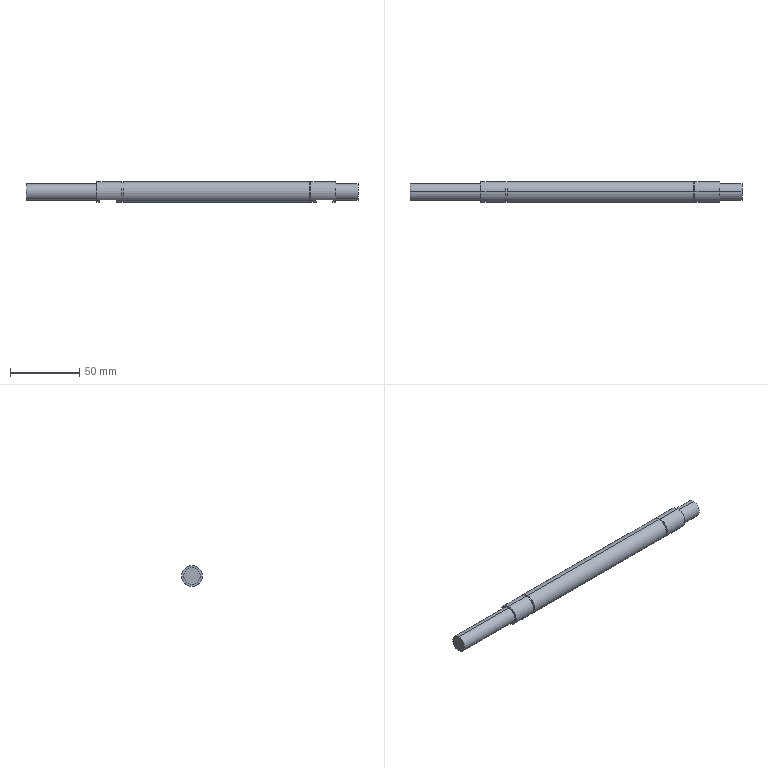Part | STEP file | MT-COMBO-119-S015 | 1 solid | 28 faces | box 239 x 15 x 15 mm | volume 37577 mm3 | cylinder 14 | plane 14 | commonest cylinder face diameters 15 x6 12 x4 13.8 x4
STEP:
#1=CARTESIAN_POINT('',(86.,0.,-6.));
#2=VERTEX_POINT('',#1);
#3=CARTESIAN_POINT('',(86.,0.,6.));
#4=VERTEX_POINT('',#3);
#5=CARTESIAN_POINT('',(86.,0.,0.));
#6=DIRECTION('',(-1.,0.,0.));
#7=DIRECTION('',(0.,0.,1.));
#8=AXIS2_PLACEMENT_3D('',#5,#6,#7);
#9=CIRCLE('',#8,6.);
#10=EDGE_CURVE('',#2,#4,#9,.T.);
#11=ORIENTED_EDGE('',*,*,#10,.F.);
#12=CARTESIAN_POINT('',(102.,0.,-6.));
#13=VERTEX_POINT('',#12);
#14=CARTESIAN_POINT('',(0.,0.,-6.));
#15=DIRECTION('',(1.,0.,0.));
#16=VECTOR('',#15,1000.);
#17=LINE('',#14,#16);
#18=EDGE_CURVE('',#2,#13,#17,.T.);
#19=ORIENTED_EDGE('',*,*,#18,.T.);
#20=CARTESIAN_POINT('',(102.,0.,6.));
#21=VERTEX_POINT('',#20);
#22=CARTESIAN_POINT('',(102.,0.,0.));
#23=DIRECTION('',(-1.,0.,0.));
#24=DIRECTION('',(0.,0.,1.));
#25=AXIS2_PLACEMENT_3D('',#22,#23,#24);
#26=CIRCLE('',#25,6.);
#27=EDGE_CURVE('',#13,#21,#26,.T.);
#28=ORIENTED_EDGE('',*,*,#27,.T.);
#29=CARTESIAN_POINT('',(0.,0.,6.));
#30=DIRECTION('',(1.,0.,0.));
#31=VECTOR('',#30,1000.);
#32=LINE('',#29,#31);
#33=EDGE_CURVE('',#4,#21,#32,.T.);
#34=ORIENTED_EDGE('',*,*,#33,.F.);
#35=EDGE_LOOP('',(#11,#19,#28,#34));
#36=FACE_OUTER_BOUND('',#35,.T.);
#37=CARTESIAN_POINT('',(0.,0.,0.));
#38=DIRECTION('',(1.,0.,0.));
#39=DIRECTION('',(0.,0.,1.));
#40=AXIS2_PLACEMENT_3D('',#37,#38,#39);
#41=CYLINDRICAL_SURFACE('',#40,6.);
#42=ADVANCED_FACE('',(#36),#41,.T.);
#43=CARTESIAN_POINT('',(68.1,0.,-6.9));
#44=VERTEX_POINT('',#43);
#45=CARTESIAN_POINT('',(68.1,0.,6.9));
#46=VERTEX_POINT('',#45);
#47=CARTESIAN_POINT('',(68.1,0.,0.));
#48=DIRECTION('',(1.,0.,0.));
#49=DIRECTION('',(0.,0.,-1.));
#50=AXIS2_PLACEMENT_3D('',#47,#48,#49);
#51=CIRCLE('',#50,6.9);
#52=EDGE_CURVE('',#44,#46,#51,.T.);
#53=ORIENTED_EDGE('',*,*,#52,.F.);
#54=CARTESIAN_POINT('',(67.,0.,-6.9));
#55=VERTEX_POINT('',#54);
#56=CARTESIAN_POINT('',(68.1,0.,-6.9));
#57=DIRECTION('',(-1.,0.,0.));
#58=VECTOR('',#57,1000.);
#59=LINE('',#56,#58);
#60=EDGE_CURVE('',#44,#55,#59,.T.);
#61=ORIENTED_EDGE('',*,*,#60,.T.);
#62=CARTESIAN_POINT('',(67.,0.,6.9));
#63=VERTEX_POINT('',#62);
#64=CARTESIAN_POINT('',(67.,0.,0.));
#65=DIRECTION('',(1.,0.,0.));
#66=DIRECTION('',(0.,0.,-1.));
#67=AXIS2_PLACEMENT_3D('',#64,#65,#66);
#68=CIRCLE('',#67,6.9);
#69=EDGE_CURVE('',#55,#63,#68,.T.);
#70=ORIENTED_EDGE('',*,*,#69,.T.);
#71=CARTESIAN_POINT('',(68.1,0.,6.9));
#72=DIRECTION('',(-1.,0.,0.));
#73=VECTOR('',#72,1000.);
#74=LINE('',#71,#73);
#75=EDGE_CURVE('',#46,#63,#74,.T.);
#76=ORIENTED_EDGE('',*,*,#75,.F.);
#77=EDGE_LOOP('',(#53,#61,#70,#76));
#78=FACE_OUTER_BOUND('',#77,.T.);
#79=CARTESIAN_POINT('',(68.1,0.,0.));
#80=DIRECTION('',(-1.,0.,0.));
#81=DIRECTION('',(0.,0.,1.));
#82=AXIS2_PLACEMENT_3D('',#79,#80,#81);
#83=CYLINDRICAL_SURFACE('',#82,6.9);
#84=ADVANCED_FACE('',(#78),#83,.T.);
#85=CARTESIAN_POINT('',(-68.1,0.,6.9));
#86=VERTEX_POINT('',#85);
#87=CARTESIAN_POINT('',(-68.1,0.,-6.9));
#88=VERTEX_POINT('',#87);
#89=CARTESIAN_POINT('',(-68.1,0.,0.));
#90=DIRECTION('',(-1.,0.,0.));
#91=DIRECTION('',(0.,0.,1.));
#92=AXIS2_PLACEMENT_3D('',#89,#90,#91);
#93=CIRCLE('',#92,6.9);
#94=EDGE_CURVE('',#86,#88,#93,.T.);
#95=ORIENTED_EDGE('',*,*,#94,.F.);
#96=CARTESIAN_POINT('',(-67.,0.,6.9));
#97=VERTEX_POINT('',#96);
#98=CARTESIAN_POINT('',(-68.1,0.,6.9));
#99=DIRECTION('',(1.,0.,0.));
#100=VECTOR('',#99,1000.);
#101=LINE('',#98,#100);
#102=EDGE_CURVE('',#86,#97,#101,.T.);
#103=ORIENTED_EDGE('',*,*,#102,.T.);
#104=CARTESIAN_POINT('',(-67.,0.,-6.9));
#105=VERTEX_POINT('',#104);
#106=CARTESIAN_POINT('',(-67.,0.,0.));
#107=DIRECTION('',(-1.,0.,0.));
#108=DIRECTION('',(0.,0.,1.));
#109=AXIS2_PLACEMENT_3D('',#106,#107,#108);
#110=CIRCLE('',#109,6.9);
#111=EDGE_CURVE('',#97,#105,#110,.T.);
#112=ORIENTED_EDGE('',*,*,#111,.T.);
#113=CARTESIAN_POINT('',(-68.1,0.,-6.9));
#114=DIRECTION('',(1.,0.,0.));
#115=VECTOR('',#114,1000.);
#116=LINE('',#113,#115);
#117=EDGE_CURVE('',#88,#105,#116,.T.);
#118=ORIENTED_EDGE('',*,*,#117,.F.);
#119=EDGE_LOOP('',(#95,#103,#112,#118));
#120=FACE_OUTER_BOUND('',#119,.T.);
#121=CARTESIAN_POINT('',(-68.1,0.,0.));
#122=DIRECTION('',(1.,0.,0.));
#123=DIRECTION('',(0.,0.,-1.));
#124=AXIS2_PLACEMENT_3D('',#121,#122,#123);
#125=CYLINDRICAL_SURFACE('',#124,6.9);
#126=ADVANCED_FACE('',(#120),#125,.T.);
#127=CARTESIAN_POINT('',(-137.,0.,-6.));
#128=VERTEX_POINT('',#127);
#129=CARTESIAN_POINT('',(-137.,0.,6.));
#130=VERTEX_POINT('',#129);
#131=CARTESIAN_POINT('',(-137.,0.,0.));
#132=DIRECTION('',(-1.,0.,0.));
#133=DIRECTION('',(0.,0.,1.));
#134=AXIS2_PLACEMENT_3D('',#131,#132,#133);
#135=CIRCLE('',#134,6.);
#136=EDGE_CURVE('',#128,#130,#135,.T.);
#137=ORIENTED_EDGE('',*,*,#136,.F.);
#138=CARTESIAN_POINT('',(-86.,0.,-6.));
#139=VERTEX_POINT('',#138);
#140=CARTESIAN_POINT('',(0.,0.,-6.));
#141=DIRECTION('',(1.,0.,0.));
#142=VECTOR('',#141,1000.);
#143=LINE('',#140,#142);
#144=EDGE_CURVE('',#128,#139,#143,.T.);
#145=ORIENTED_EDGE('',*,*,#144,.T.);
#146=CARTESIAN_POINT('',(-86.,0.,6.));
#147=VERTEX_POINT('',#146);
#148=CARTESIAN_POINT('',(-86.,0.,0.));
#149=DIRECTION('',(-1.,0.,0.));
#150=DIRECTION('',(0.,0.,1.));
#151=AXIS2_PLACEMENT_3D('',#148,#149,#150);
#152=CIRCLE('',#151,6.);
#153=EDGE_CURVE('',#139,#147,#152,.T.);
#154=ORIENTED_EDGE('',*,*,#153,.T.);
#155=CARTESIAN_POINT('',(0.,0.,6.));
#156=DIRECTION('',(1.,0.,0.));
#157=VECTOR('',#156,1000.);
#158=LINE('',#155,#157);
#159=EDGE_CURVE('',#130,#147,#158,.T.);
#160=ORIENTED_EDGE('',*,*,#159,.F.);
#161=EDGE_LOOP('',(#137,#145,#154,#160));
#162=FACE_OUTER_BOUND('',#161,.T.);
#163=CARTESIAN_POINT('',(0.,0.,0.));
#164=DIRECTION('',(1.,0.,0.));
#165=DIRECTION('',(0.,0.,1.));
#166=AXIS2_PLACEMENT_3D('',#163,#164,#165);
#167=CYLINDRICAL_SURFACE('',#166,6.);
#168=ADVANCED_FACE('',(#162),#167,.T.);
#169=CARTESIAN_POINT('',(67.,0.,-7.5));
#170=VERTEX_POINT('',#169);
#171=CARTESIAN_POINT('',(67.,0.,7.5));
#172=VERTEX_POINT('',#171);
#173=CARTESIAN_POINT('',(67.,0.,0.));
#174=DIRECTION('',(1.,0.,0.));
#175=DIRECTION('',(0.,0.,-1.));
#176=AXIS2_PLACEMENT_3D('',#173,#174,#175);
#177=CIRCLE('',#176,7.5);
#178=EDGE_CURVE('',#170,#172,#177,.T.);
#179=ORIENTED_EDGE('',*,*,#178,.F.);
#180=CARTESIAN_POINT('',(-67.,0.,-7.5));
#181=VERTEX_POINT('',#180);
#182=CARTESIAN_POINT('',(107.213,0.,-7.5));
#183=DIRECTION('',(-1.,0.,0.));
#184=VECTOR('',#183,1000.);
#185=LINE('',#182,#184);
#186=EDGE_CURVE('',#170,#181,#185,.T.);
#187=ORIENTED_EDGE('',*,*,#186,.T.);
#188=CARTESIAN_POINT('',(-67.,0.,7.5));
#189=VERTEX_POINT('',#188);
#190=CARTESIAN_POINT('',(-67.,0.,0.));
#191=DIRECTION('',(-1.,0.,0.));
#192=DIRECTION('',(0.,0.,1.));
#193=AXIS2_PLACEMENT_3D('',#190,#191,#192);
#194=CIRCLE('',#193,7.5);
#195=EDGE_CURVE('',#189,#181,#194,.T.);
#196=ORIENTED_EDGE('',*,*,#195,.F.);
#197=CARTESIAN_POINT('',(107.213,0.,7.5));
#198=DIRECTION('',(-1.,0.,0.));
#199=VECTOR('',#198,1000.);
#200=LINE('',#197,#199);
#201=EDGE_CURVE('',#172,#189,#200,.T.);
#202=ORIENTED_EDGE('',*,*,#201,.F.);
#203=EDGE_LOOP('',(#179,#187,#196,#202));
#204=FACE_OUTER_BOUND('',#203,.T.);
#205=CARTESIAN_POINT('',(107.213,0.,0.));
#206=DIRECTION('',(-1.,0.,0.));
#207=DIRECTION('',(0.,0.,1.));
#208=AXIS2_PLACEMENT_3D('',#205,#206,#207);
#209=CYLINDRICAL_SURFACE('',#208,7.5);
#210=ADVANCED_FACE('',(#204),#209,.T.);
#211=CARTESIAN_POINT('',(-68.1,0.,7.5));
#212=VERTEX_POINT('',#211);
#213=CARTESIAN_POINT('',(-68.1,0.,-7.5));
#214=VERTEX_POINT('',#213);
#215=CARTESIAN_POINT('',(-68.1,0.,0.));
#216=DIRECTION('',(-1.,0.,0.));
#217=DIRECTION('',(0.,0.,1.));
#218=AXIS2_PLACEMENT_3D('',#215,#216,#217);
#219=CIRCLE('',#218,7.5);
#220=EDGE_CURVE('',#212,#214,#219,.T.);
#221=ORIENTED_EDGE('',*,*,#220,.T.);
#222=CARTESIAN_POINT('',(-72.,0.,-7.5));
#223=VERTEX_POINT('',#222);
#224=CARTESIAN_POINT('',(107.213,0.,-7.5));
#225=DIRECTION('',(-1.,0.,0.));
#226=VECTOR('',#225,1000.);
#227=LINE('',#224,#226);
#228=EDGE_CURVE('',#214,#223,#227,.T.);
#229=ORIENTED_EDGE('',*,*,#228,.T.);
#230=CARTESIAN_POINT('',(-72.,5.099,-5.5));
#231=VERTEX_POINT('',#230);
#232=CARTESIAN_POINT('',(-72.,0.,0.));
#233=DIRECTION('',(-1.,0.,0.));
#234=DIRECTION('',(0.,0.,-1.));
#235=AXIS2_PLACEMENT_3D('',#232,#233,#234);
#236=CIRCLE('',#235,7.5);
#237=EDGE_CURVE('',#231,#223,#236,.T.);
#238=ORIENTED_EDGE('',*,*,#237,.F.);
#239=CARTESIAN_POINT('',(-84.,5.099,-5.5));
#240=VERTEX_POINT('',#239);
#241=CARTESIAN_POINT('',(107.213,5.099,-5.5));
#242=DIRECTION('',(-1.,0.,0.));
#243=VECTOR('',#242,1000.);
#244=LINE('',#241,#243);
#245=EDGE_CURVE('',#231,#240,#244,.T.);
#246=ORIENTED_EDGE('',*,*,#245,.T.);
#247=CARTESIAN_POINT('',(-84.,0.,-7.5));
#248=VERTEX_POINT('',#247);
#249=CARTESIAN_POINT('',(-84.,0.,0.));
#250=DIRECTION('',(1.,0.,0.));
#251=DIRECTION('',(0.,0.,1.));
#252=AXIS2_PLACEMENT_3D('',#249,#250,#251);
#253=CIRCLE('',#252,7.5);
#254=EDGE_CURVE('',#248,#240,#253,.T.);
#255=ORIENTED_EDGE('',*,*,#254,.F.);
#256=CARTESIAN_POINT('',(-86.,0.,-7.5));
#257=VERTEX_POINT('',#256);
#258=CARTESIAN_POINT('',(107.213,0.,-7.5));
#259=DIRECTION('',(-1.,0.,0.));
#260=VECTOR('',#259,1000.);
#261=LINE('',#258,#260);
#262=EDGE_CURVE('',#248,#257,#261,.T.);
#263=ORIENTED_EDGE('',*,*,#262,.T.);
#264=CARTESIAN_POINT('',(-86.,0.,7.5));
#265=VERTEX_POINT('',#264);
#266=CARTESIAN_POINT('',(-86.,0.,0.));
#267=DIRECTION('',(-1.,0.,0.));
#268=DIRECTION('',(0.,0.,1.));
#269=AXIS2_PLACEMENT_3D('',#266,#267,#268);
#270=CIRCLE('',#269,7.5);
#271=EDGE_CURVE('',#265,#257,#270,.T.);
#272=ORIENTED_EDGE('',*,*,#271,.F.);
#273=CARTESIAN_POINT('',(107.213,0.,7.5));
#274=DIRECTION('',(-1.,0.,0.));
#275=VECTOR('',#274,1000.);
#276=LINE('',#273,#275);
#277=EDGE_CURVE('',#212,#265,#276,.T.);
#278=ORIENTED_EDGE('',*,*,#277,.F.);
#279=EDGE_LOOP('',(#221,#229,#238,#246,#255,#263,#272,#278));
#280=FACE_OUTER_BOUND('',#279,.T.);
#281=CARTESIAN_POINT('',(107.213,0.,0.));
#282=DIRECTION('',(-1.,0.,0.));
#283=DIRECTION('',(0.,0.,1.));
#284=AXIS2_PLACEMENT_3D('',#281,#282,#283);
#285=CYLINDRICAL_SURFACE('',#284,7.5);
#286=ADVANCED_FACE('',(#280),#285,.T.);
#287=CARTESIAN_POINT('',(86.,0.,7.5));
#288=VERTEX_POINT('',#287);
#289=CARTESIAN_POINT('',(86.,0.,-7.5));
#290=VERTEX_POINT('',#289);
#291=CARTESIAN_POINT('',(86.,0.,0.));
#292=DIRECTION('',(-1.,0.,0.));
#293=DIRECTION('',(0.,0.,-1.));
#294=AXIS2_PLACEMENT_3D('',#291,#292,#293);
#295=CIRCLE('',#294,7.5);
#296=EDGE_CURVE('',#288,#290,#295,.T.);
#297=ORIENTED_EDGE('',*,*,#296,.T.);
#298=CARTESIAN_POINT('',(84.,0.,-7.5));
#299=VERTEX_POINT('',#298);
#300=CARTESIAN_POINT('',(107.213,0.,-7.5));
#301=DIRECTION('',(-1.,0.,0.));
#302=VECTOR('',#301,1000.);
#303=LINE('',#300,#302);
#304=EDGE_CURVE('',#290,#299,#303,.T.);
#305=ORIENTED_EDGE('',*,*,#304,.T.);
#306=CARTESIAN_POINT('',(84.,5.099,-5.5));
#307=VERTEX_POINT('',#306);
#308=CARTESIAN_POINT('',(84.,0.,0.));
#309=DIRECTION('',(-1.,0.,0.));
#310=DIRECTION('',(0.,0.,-1.));
#311=AXIS2_PLACEMENT_3D('',#308,#309,#310);
#312=CIRCLE('',#311,7.5);
#313=EDGE_CURVE('',#307,#299,#312,.T.);
#314=ORIENTED_EDGE('',*,*,#313,.F.);
#315=CARTESIAN_POINT('',(72.,5.099,-5.5));
#316=VERTEX_POINT('',#315);
#317=CARTESIAN_POINT('',(107.213,5.099,-5.5));
#318=DIRECTION('',(-1.,0.,0.));
#319=VECTOR('',#318,1000.);
#320=LINE('',#317,#319);
#321=EDGE_CURVE('',#307,#316,#320,.T.);
#322=ORIENTED_EDGE('',*,*,#321,.T.);
#323=CARTESIAN_POINT('',(72.,0.,-7.5));
#324=VERTEX_POINT('',#323);
#325=CARTESIAN_POINT('',(72.,0.,0.));
#326=DIRECTION('',(1.,0.,0.));
#327=DIRECTION('',(0.,0.,1.));
#328=AXIS2_PLACEMENT_3D('',#325,#326,#327);
#329=CIRCLE('',#328,7.5);
#330=EDGE_CURVE('',#324,#316,#329,.T.);
#331=ORIENTED_EDGE('',*,*,#330,.F.);
#332=CARTESIAN_POINT('',(68.1,0.,-7.5));
#333=VERTEX_POINT('',#332);
#334=CARTESIAN_POINT('',(107.213,0.,-7.5));
#335=DIRECTION('',(-1.,0.,0.));
#336=VECTOR('',#335,1000.);
#337=LINE('',#334,#336);
#338=EDGE_CURVE('',#324,#333,#337,.T.);
#339=ORIENTED_EDGE('',*,*,#338,.T.);
#340=CARTESIAN_POINT('',(68.1,0.,7.5));
#341=VERTEX_POINT('',#340);
#342=CARTESIAN_POINT('',(68.1,0.,0.));
#343=DIRECTION('',(1.,0.,0.));
#344=DIRECTION('',(0.,0.,-1.));
#345=AXIS2_PLACEMENT_3D('',#342,#343,#344);
#346=CIRCLE('',#345,7.5);
#347=EDGE_CURVE('',#333,#341,#346,.T.);
#348=ORIENTED_EDGE('',*,*,#347,.T.);
#349=CARTESIAN_POINT('',(107.213,0.,7.5));
#350=DIRECTION('',(-1.,0.,0.));
#351=VECTOR('',#350,1000.);
#352=LINE('',#349,#351);
#353=EDGE_CURVE('',#288,#341,#352,.T.);
#354=ORIENTED_EDGE('',*,*,#353,.F.);
#355=EDGE_LOOP('',(#297,#305,#314,#322,#331,#339,#348,#354));
#356=FACE_OUTER_BOUND('',#355,.T.);
#357=CARTESIAN_POINT('',(107.213,0.,0.));
#358=DIRECTION('',(-1.,0.,0.));
#359=DIRECTION('',(0.,0.,1.));
#360=AXIS2_PLACEMENT_3D('',#357,#358,#359);
#361=CYLINDRICAL_SURFACE('',#360,7.5);
#362=ADVANCED_FACE('',(#356),#361,.T.);
#363=ORIENTED_EDGE('',*,*,#304,.F.);
#364=CARTESIAN_POINT('',(86.,0.,0.));
#365=DIRECTION('',(-1.,0.,0.));
#366=DIRECTION('',(0.,0.,-1.));
#367=AXIS2_PLACEMENT_3D('',#364,#365,#366);
#368=CIRCLE('',#367,7.5);
#369=EDGE_CURVE('',#290,#288,#368,.T.);
#370=ORIENTED_EDGE('',*,*,#369,.T.);
#371=ORIENTED_EDGE('',*,*,#353,.T.);
#372=CARTESIAN_POINT('',(68.1,0.,0.));
#373=DIRECTION('',(1.,0.,0.));
#374=DIRECTION('',(0.,0.,-1.));
#375=AXIS2_PLACEMENT_3D('',#372,#373,#374);
#376=CIRCLE('',#375,7.5);
#377=EDGE_CURVE('',#341,#333,#376,.T.);
#378=ORIENTED_EDGE('',*,*,#377,.T.);
#379=ORIENTED_EDGE('',*,*,#338,.F.);
#380=CARTESIAN_POINT('',(72.,-5.099,-5.5));
#381=VERTEX_POINT('',#380);
#382=CARTESIAN_POINT('',(72.,0.,0.));
#383=DIRECTION('',(1.,0.,0.));
#384=DIRECTION('',(0.,0.,1.));
#385=AXIS2_PLACEMENT_3D('',#382,#383,#384);
#386=CIRCLE('',#385,7.5);
#387=EDGE_CURVE('',#381,#324,#386,.T.);
#388=ORIENTED_EDGE('',*,*,#387,.F.);
#389=CARTESIAN_POINT('',(84.,-5.099,-5.5));
#390=VERTEX_POINT('',#389);
#391=CARTESIAN_POINT('',(107.213,-5.099,-5.5));
#392=DIRECTION('',(1.,0.,0.));
#393=VECTOR('',#392,1000.);
#394=LINE('',#391,#393);
#395=EDGE_CURVE('',#381,#390,#394,.T.);
#396=ORIENTED_EDGE('',*,*,#395,.T.);
#397=CARTESIAN_POINT('',(84.,0.,0.));
#398=DIRECTION('',(-1.,0.,0.));
#399=DIRECTION('',(0.,0.,-1.));
#400=AXIS2_PLACEMENT_3D('',#397,#398,#399);
#401=CIRCLE('',#400,7.5);
#402=EDGE_CURVE('',#299,#390,#401,.T.);
#403=ORIENTED_EDGE('',*,*,#402,.F.);
#404=EDGE_LOOP('',(#363,#370,#371,#378,#379,#388,#396,#403));
#405=FACE_OUTER_BOUND('',#404,.T.);
#406=CARTESIAN_POINT('',(107.213,0.,0.));
#407=DIRECTION('',(-1.,0.,0.));
#408=DIRECTION('',(0.,0.,1.));
#409=AXIS2_PLACEMENT_3D('',#406,#407,#408);
#410=CYLINDRICAL_SURFACE('',#409,7.5);
#411=ADVANCED_FACE('',(#405),#410,.T.);
#412=ORIENTED_EDGE('',*,*,#228,.F.);
#413=CARTESIAN_POINT('',(-68.1,0.,0.));
#414=DIRECTION('',(-1.,0.,0.));
#415=DIRECTION('',(0.,0.,1.));
#416=AXIS2_PLACEMENT_3D('',#413,#414,#415);
#417=CIRCLE('',#416,7.5);
#418=EDGE_CURVE('',#214,#212,#417,.T.);
#419=ORIENTED_EDGE('',*,*,#418,.T.);
#420=ORIENTED_EDGE('',*,*,#277,.T.);
#421=CARTESIAN_POINT('',(-86.,0.,0.));
#422=DIRECTION('',(-1.,0.,0.));
#423=DIRECTION('',(0.,0.,1.));
#424=AXIS2_PLACEMENT_3D('',#421,#422,#423);
#425=CIRCLE('',#424,7.5);
#426=EDGE_CURVE('',#257,#265,#425,.T.);
#427=ORIENTED_EDGE('',*,*,#426,.F.);
#428=ORIENTED_EDGE('',*,*,#262,.F.);
#429=CARTESIAN_POINT('',(-84.,-5.099,-5.5));
#430=VERTEX_POINT('',#429);
#431=CARTESIAN_POINT('',(-84.,0.,0.));
#432=DIRECTION('',(1.,0.,0.));
#433=DIRECTION('',(0.,0.,1.));
#434=AXIS2_PLACEMENT_3D('',#431,#432,#433);
#435=CIRCLE('',#434,7.5);
#436=EDGE_CURVE('',#430,#248,#435,.T.);
#437=ORIENTED_EDGE('',*,*,#436,.F.);
#438=CARTESIAN_POINT('',(-72.,-5.099,-5.5));
#439=VERTEX_POINT('',#438);
#440=CARTESIAN_POINT('',(107.213,-5.099,-5.5));
#441=DIRECTION('',(1.,0.,0.));
#442=VECTOR('',#441,1000.);
#443=LINE('',#440,#442);
#444=EDGE_CURVE('',#430,#439,#443,.T.);
#445=ORIENTED_EDGE('',*,*,#444,.T.);
#446=CARTESIAN_POINT('',(-72.,0.,0.));
#447=DIRECTION('',(-1.,0.,0.));
#448=DIRECTION('',(0.,0.,-1.));
#449=AXIS2_PLACEMENT_3D('',#446,#447,#448);
#450=CIRCLE('',#449,7.5);
#451=EDGE_CURVE('',#223,#439,#450,.T.);
#452=ORIENTED_EDGE('',*,*,#451,.F.);
#453=EDGE_LOOP('',(#412,#419,#420,#427,#428,#437,#445,#452));
#454=FACE_OUTER_BOUND('',#453,.T.);
#455=CARTESIAN_POINT('',(107.213,0.,0.));
#456=DIRECTION('',(-1.,0.,0.));
#457=DIRECTION('',(0.,0.,1.));
#458=AXIS2_PLACEMENT_3D('',#455,#456,#457);
#459=CYLINDRICAL_SURFACE('',#458,7.5);
#460=ADVANCED_FACE('',(#454),#459,.T.);
#461=ORIENTED_EDGE('',*,*,#186,.F.);
#462=CARTESIAN_POINT('',(67.,0.,0.));
#463=DIRECTION('',(1.,0.,0.));
#464=DIRECTION('',(0.,0.,-1.));
#465=AXIS2_PLACEMENT_3D('',#462,#463,#464);
#466=CIRCLE('',#465,7.5);
#467=EDGE_CURVE('',#172,#170,#466,.T.);
#468=ORIENTED_EDGE('',*,*,#467,.F.);
#469=ORIENTED_EDGE('',*,*,#201,.T.);
#470=CARTESIAN_POINT('',(-67.,0.,0.));
#471=DIRECTION('',(-1.,0.,0.));
#472=DIRECTION('',(0.,0.,1.));
#473=AXIS2_PLACEMENT_3D('',#470,#471,#472);
#474=CIRCLE('',#473,7.5);
#475=EDGE_CURVE('',#181,#189,#474,.T.);
#476=ORIENTED_EDGE('',*,*,#475,.F.);
#477=EDGE_LOOP('',(#461,#468,#469,#476));
#478=FACE_OUTER_BOUND('',#477,.T.);
#479=CARTESIAN_POINT('',(107.213,0.,0.));
#480=DIRECTION('',(-1.,0.,0.));
#481=DIRECTION('',(0.,0.,1.));
#482=AXIS2_PLACEMENT_3D('',#479,#480,#481);
#483=CYLINDRICAL_SURFACE('',#482,7.5);
#484=ADVANCED_FACE('',(#478),#483,.T.);
#485=CARTESIAN_POINT('',(-137.,0.,0.));
#486=DIRECTION('',(-1.,0.,0.));
#487=DIRECTION('',(0.,0.,1.));
#488=AXIS2_PLACEMENT_3D('',#485,#486,#487);
#489=CIRCLE('',#488,6.);
#490=EDGE_CURVE('',#130,#128,#489,.T.);
#491=ORIENTED_EDGE('',*,*,#490,.T.);
#492=ORIENTED_EDGE('',*,*,#136,.T.);
#493=EDGE_LOOP('',(#491,#492));
#494=FACE_OUTER_BOUND('',#493,.T.);
#495=CARTESIAN_POINT('',(-137.,0.,0.));
#496=DIRECTION('',(-1.,0.,0.));
#497=DIRECTION('',(0.,0.,-1.));
#498=AXIS2_PLACEMENT_3D('',#495,#496,#497);
#499=PLANE('',#498);
#500=ADVANCED_FACE('',(#494),#499,.T.);
#501=ORIENTED_EDGE('',*,*,#144,.F.);
#502=ORIENTED_EDGE('',*,*,#490,.F.);
#503=ORIENTED_EDGE('',*,*,#159,.T.);
#504=CARTESIAN_POINT('',(-86.,0.,0.));
#505=DIRECTION('',(-1.,0.,0.));
#506=DIRECTION('',(0.,0.,1.));
#507=AXIS2_PLACEMENT_3D('',#504,#505,#506);
#508=CIRCLE('',#507,6.);
#509=EDGE_CURVE('',#147,#139,#508,.T.);
#510=ORIENTED_EDGE('',*,*,#509,.T.);
#511=EDGE_LOOP('',(#501,#502,#503,#510));
#512=FACE_OUTER_BOUND('',#511,.T.);
#513=CARTESIAN_POINT('',(0.,0.,0.));
#514=DIRECTION('',(1.,0.,0.));
#515=DIRECTION('',(0.,0.,1.));
#516=AXIS2_PLACEMENT_3D('',#513,#514,#515);
#517=CYLINDRICAL_SURFACE('',#516,6.);
#518=ADVANCED_FACE('',(#512),#517,.T.);
#519=ORIENTED_EDGE('',*,*,#509,.F.);
#520=ORIENTED_EDGE('',*,*,#153,.F.);
#521=EDGE_LOOP('',(#519,#520));
#522=FACE_BOUND('',#521,.T.);
#523=ORIENTED_EDGE('',*,*,#271,.T.);
#524=ORIENTED_EDGE('',*,*,#426,.T.);
#525=EDGE_LOOP('',(#523,#524));
#526=FACE_OUTER_BOUND('',#525,.T.);
#527=CARTESIAN_POINT('',(-86.,7.,0.));
#528=DIRECTION('',(-1.,0.,0.));
#529=DIRECTION('',(0.,0.,-1.));
#530=AXIS2_PLACEMENT_3D('',#527,#528,#529);
#531=PLANE('',#530);
#532=ADVANCED_FACE('',(#522,#526),#531,.T.);
#533=ORIENTED_EDGE('',*,*,#220,.F.);
#534=ORIENTED_EDGE('',*,*,#418,.F.);
#535=EDGE_LOOP('',(#533,#534));
#536=FACE_OUTER_BOUND('',#535,.T.);
#537=CARTESIAN_POINT('',(-68.1,0.,0.));
#538=DIRECTION('',(-1.,0.,0.));
#539=DIRECTION('',(0.,0.,1.));
#540=AXIS2_PLACEMENT_3D('',#537,#538,#539);
#541=CIRCLE('',#540,6.9);
#542=EDGE_CURVE('',#88,#86,#541,.T.);
#543=ORIENTED_EDGE('',*,*,#542,.T.);
#544=ORIENTED_EDGE('',*,*,#94,.T.);
#545=EDGE_LOOP('',(#543,#544));
#546=FACE_BOUND('',#545,.T.);
#547=CARTESIAN_POINT('',(-68.1,0.,0.));
#548=DIRECTION('',(-1.,0.,0.));
#549=DIRECTION('',(0.,0.,1.));
#550=AXIS2_PLACEMENT_3D('',#547,#548,#549);
#551=PLANE('',#550);
#552=ADVANCED_FACE('',(#536,#546),#551,.F.);
#553=ORIENTED_EDGE('',*,*,#195,.T.);
#554=ORIENTED_EDGE('',*,*,#475,.T.);
#555=EDGE_LOOP('',(#553,#554));
#556=FACE_OUTER_BOUND('',#555,.T.);
#557=CARTESIAN_POINT('',(-67.,0.,0.));
#558=DIRECTION('',(-1.,0.,0.));
#559=DIRECTION('',(0.,0.,1.));
#560=AXIS2_PLACEMENT_3D('',#557,#558,#559);
#561=CIRCLE('',#560,6.9);
#562=EDGE_CURVE('',#105,#97,#561,.T.);
#563=ORIENTED_EDGE('',*,*,#562,.F.);
#564=ORIENTED_EDGE('',*,*,#111,.F.);
#565=EDGE_LOOP('',(#563,#564));
#566=FACE_BOUND('',#565,.T.);
#567=CARTESIAN_POINT('',(-67.,0.,0.));
#568=DIRECTION('',(-1.,0.,0.));
#569=DIRECTION('',(0.,0.,1.));
#570=AXIS2_PLACEMENT_3D('',#567,#568,#569);
#571=PLANE('',#570);
#572=ADVANCED_FACE('',(#556,#566),#571,.T.);
#573=ORIENTED_EDGE('',*,*,#102,.F.);
#574=ORIENTED_EDGE('',*,*,#542,.F.);
#575=ORIENTED_EDGE('',*,*,#117,.T.);
#576=ORIENTED_EDGE('',*,*,#562,.T.);
#577=EDGE_LOOP('',(#573,#574,#575,#576));
#578=FACE_OUTER_BOUND('',#577,.T.);
#579=CARTESIAN_POINT('',(-68.1,0.,0.));
#580=DIRECTION('',(1.,0.,0.));
#581=DIRECTION('',(0.,0.,-1.));
#582=AXIS2_PLACEMENT_3D('',#579,#580,#581);
#583=CYLINDRICAL_SURFACE('',#582,6.9);
#584=ADVANCED_FACE('',(#578),#583,.T.);
#585=ORIENTED_EDGE('',*,*,#377,.F.);
#586=ORIENTED_EDGE('',*,*,#347,.F.);
#587=EDGE_LOOP('',(#585,#586));
#588=FACE_OUTER_BOUND('',#587,.T.);
#589=CARTESIAN_POINT('',(68.1,0.,0.));
#590=DIRECTION('',(1.,0.,0.));
#591=DIRECTION('',(0.,0.,-1.));
#592=AXIS2_PLACEMENT_3D('',#589,#590,#591);
#593=CIRCLE('',#592,6.9);
#594=EDGE_CURVE('',#46,#44,#593,.T.);
#595=ORIENTED_EDGE('',*,*,#594,.T.);
#596=ORIENTED_EDGE('',*,*,#52,.T.);
#597=EDGE_LOOP('',(#595,#596));
#598=FACE_BOUND('',#597,.T.);
#599=CARTESIAN_POINT('',(68.1,0.,0.));
#600=DIRECTION('',(1.,0.,0.));
#601=DIRECTION('',(0.,0.,-1.));
#602=AXIS2_PLACEMENT_3D('',#599,#600,#601);
#603=PLANE('',#602);
#604=ADVANCED_FACE('',(#588,#598),#603,.F.);
#605=ORIENTED_EDGE('',*,*,#467,.T.);
#606=ORIENTED_EDGE('',*,*,#178,.T.);
#607=EDGE_LOOP('',(#605,#606));
#608=FACE_OUTER_BOUND('',#607,.T.);
#609=CARTESIAN_POINT('',(67.,0.,0.));
#610=DIRECTION('',(1.,0.,0.));
#611=DIRECTION('',(0.,0.,-1.));
#612=AXIS2_PLACEMENT_3D('',#609,#610,#611);
#613=CIRCLE('',#612,6.9);
#614=EDGE_CURVE('',#63,#55,#613,.T.);
#615=ORIENTED_EDGE('',*,*,#614,.F.);
#616=ORIENTED_EDGE('',*,*,#69,.F.);
#617=EDGE_LOOP('',(#615,#616));
#618=FACE_BOUND('',#617,.T.);
#619=CARTESIAN_POINT('',(67.,0.,0.));
#620=DIRECTION('',(1.,0.,0.));
#621=DIRECTION('',(0.,0.,-1.));
#622=AXIS2_PLACEMENT_3D('',#619,#620,#621);
#623=PLANE('',#622);
#624=ADVANCED_FACE('',(#608,#618),#623,.T.);
#625=ORIENTED_EDGE('',*,*,#60,.F.);
#626=ORIENTED_EDGE('',*,*,#594,.F.);
#627=ORIENTED_EDGE('',*,*,#75,.T.);
#628=ORIENTED_EDGE('',*,*,#614,.T.);
#629=EDGE_LOOP('',(#625,#626,#627,#628));
#630=FACE_OUTER_BOUND('',#629,.T.);
#631=CARTESIAN_POINT('',(68.1,0.,0.));
#632=DIRECTION('',(-1.,0.,0.));
#633=DIRECTION('',(0.,0.,1.));
#634=AXIS2_PLACEMENT_3D('',#631,#632,#633);
#635=CYLINDRICAL_SURFACE('',#634,6.9);
#636=ADVANCED_FACE('',(#630),#635,.T.);
#637=CARTESIAN_POINT('',(102.,0.,0.));
#638=DIRECTION('',(-1.,0.,0.));
#639=DIRECTION('',(0.,0.,1.));
#640=AXIS2_PLACEMENT_3D('',#637,#638,#639);
#641=CIRCLE('',#640,6.);
#642=EDGE_CURVE('',#21,#13,#641,.T.);
#643=ORIENTED_EDGE('',*,*,#642,.F.);
#644=ORIENTED_EDGE('',*,*,#27,.F.);
#645=EDGE_LOOP('',(#643,#644));
#646=FACE_OUTER_BOUND('',#645,.T.);
#647=CARTESIAN_POINT('',(102.,6.,0.));
#648=DIRECTION('',(1.,0.,0.));
#649=DIRECTION('',(0.,0.,1.));
#650=AXIS2_PLACEMENT_3D('',#647,#648,#649);
#651=PLANE('',#650);
#652=ADVANCED_FACE('',(#646),#651,.T.);
#653=ORIENTED_EDGE('',*,*,#18,.F.);
#654=CARTESIAN_POINT('',(86.,0.,0.));
#655=DIRECTION('',(-1.,0.,0.));
#656=DIRECTION('',(0.,0.,1.));
#657=AXIS2_PLACEMENT_3D('',#654,#655,#656);
#658=CIRCLE('',#657,6.);
#659=EDGE_CURVE('',#4,#2,#658,.T.);
#660=ORIENTED_EDGE('',*,*,#659,.F.);
#661=ORIENTED_EDGE('',*,*,#33,.T.);
#662=ORIENTED_EDGE('',*,*,#642,.T.);
#663=EDGE_LOOP('',(#653,#660,#661,#662));
#664=FACE_OUTER_BOUND('',#663,.T.);
#665=CARTESIAN_POINT('',(0.,0.,0.));
#666=DIRECTION('',(1.,0.,0.));
#667=DIRECTION('',(0.,0.,1.));
#668=AXIS2_PLACEMENT_3D('',#665,#666,#667);
#669=CYLINDRICAL_SURFACE('',#668,6.);
#670=ADVANCED_FACE('',(#664),#669,.T.);
#671=ORIENTED_EDGE('',*,*,#659,.T.);
#672=ORIENTED_EDGE('',*,*,#10,.T.);
#673=EDGE_LOOP('',(#671,#672));
#674=FACE_BOUND('',#673,.T.);
#675=ORIENTED_EDGE('',*,*,#296,.F.);
#676=ORIENTED_EDGE('',*,*,#369,.F.);
#677=EDGE_LOOP('',(#675,#676));
#678=FACE_OUTER_BOUND('',#677,.T.);
#679=CARTESIAN_POINT('',(86.,7.,0.));
#680=DIRECTION('',(1.,0.,0.));
#681=DIRECTION('',(0.,0.,1.));
#682=AXIS2_PLACEMENT_3D('',#679,#680,#681);
#683=PLANE('',#682);
#684=ADVANCED_FACE('',(#674,#678),#683,.T.);
#685=ORIENTED_EDGE('',*,*,#237,.T.);
#686=ORIENTED_EDGE('',*,*,#451,.T.);
#687=CARTESIAN_POINT('',(-72.,-29.291,-5.5));
#688=DIRECTION('',(0.,-1.,0.));
#689=VECTOR('',#688,1000.);
#690=LINE('',#687,#689);
#691=EDGE_CURVE('',#231,#439,#690,.T.);
#692=ORIENTED_EDGE('',*,*,#691,.F.);
#693=EDGE_LOOP('',(#685,#686,#692));
#694=FACE_OUTER_BOUND('',#693,.T.);
#695=CARTESIAN_POINT('',(-72.,-29.291,-5.5));
#696=DIRECTION('',(1.,0.,0.));
#697=DIRECTION('',(0.,0.,-1.));
#698=AXIS2_PLACEMENT_3D('',#695,#696,#697);
#699=PLANE('',#698);
#700=ADVANCED_FACE('',(#694),#699,.F.);
#701=CARTESIAN_POINT('',(-84.,-29.291,-5.5));
#702=DIRECTION('',(0.,1.,0.));
#703=VECTOR('',#702,1000.);
#704=LINE('',#701,#703);
#705=EDGE_CURVE('',#430,#240,#704,.T.);
#706=ORIENTED_EDGE('',*,*,#705,.F.);
#707=ORIENTED_EDGE('',*,*,#436,.T.);
#708=ORIENTED_EDGE('',*,*,#254,.T.);
#709=EDGE_LOOP('',(#706,#707,#708));
#710=FACE_OUTER_BOUND('',#709,.T.);
#711=CARTESIAN_POINT('',(-84.,-29.291,-5.5));
#712=DIRECTION('',(-1.,0.,0.));
#713=DIRECTION('',(0.,0.,1.));
#714=AXIS2_PLACEMENT_3D('',#711,#712,#713);
#715=PLANE('',#714);
#716=ADVANCED_FACE('',(#710),#715,.F.);
#717=ORIENTED_EDGE('',*,*,#705,.T.);
#718=ORIENTED_EDGE('',*,*,#245,.F.);
#719=ORIENTED_EDGE('',*,*,#691,.T.);
#720=ORIENTED_EDGE('',*,*,#444,.F.);
#721=EDGE_LOOP('',(#717,#718,#719,#720));
#722=FACE_OUTER_BOUND('',#721,.T.);
#723=CARTESIAN_POINT('',(0.,0.,-5.5));
#724=DIRECTION('',(0.,0.,-1.));
#725=DIRECTION('',(-1.,0.,0.));
#726=AXIS2_PLACEMENT_3D('',#723,#724,#725);
#727=PLANE('',#726);
#728=ADVANCED_FACE('',(#722),#727,.T.);
#729=ORIENTED_EDGE('',*,*,#313,.T.);
#730=ORIENTED_EDGE('',*,*,#402,.T.);
#731=CARTESIAN_POINT('',(84.,-29.291,-5.5));
#732=DIRECTION('',(0.,-1.,0.));
#733=VECTOR('',#732,1000.);
#734=LINE('',#731,#733);
#735=EDGE_CURVE('',#307,#390,#734,.T.);
#736=ORIENTED_EDGE('',*,*,#735,.F.);
#737=EDGE_LOOP('',(#729,#730,#736));
#738=FACE_OUTER_BOUND('',#737,.T.);
#739=CARTESIAN_POINT('',(84.,-29.291,-5.5));
#740=DIRECTION('',(1.,0.,0.));
#741=DIRECTION('',(0.,0.,-1.));
#742=AXIS2_PLACEMENT_3D('',#739,#740,#741);
#743=PLANE('',#742);
#744=ADVANCED_FACE('',(#738),#743,.F.);
#745=CARTESIAN_POINT('',(72.,-29.291,-5.5));
#746=DIRECTION('',(0.,1.,0.));
#747=VECTOR('',#746,1000.);
#748=LINE('',#745,#747);
#749=EDGE_CURVE('',#381,#316,#748,.T.);
#750=ORIENTED_EDGE('',*,*,#749,.F.);
#751=ORIENTED_EDGE('',*,*,#387,.T.);
#752=ORIENTED_EDGE('',*,*,#330,.T.);
#753=EDGE_LOOP('',(#750,#751,#752));
#754=FACE_OUTER_BOUND('',#753,.T.);
#755=CARTESIAN_POINT('',(72.,-29.291,-5.5));
#756=DIRECTION('',(-1.,0.,0.));
#757=DIRECTION('',(0.,0.,1.));
#758=AXIS2_PLACEMENT_3D('',#755,#756,#757);
#759=PLANE('',#758);
#760=ADVANCED_FACE('',(#754),#759,.F.);
#761=ORIENTED_EDGE('',*,*,#749,.T.);
#762=ORIENTED_EDGE('',*,*,#321,.F.);
#763=ORIENTED_EDGE('',*,*,#735,.T.);
#764=ORIENTED_EDGE('',*,*,#395,.F.);
#765=EDGE_LOOP('',(#761,#762,#763,#764));
#766=FACE_OUTER_BOUND('',#765,.T.);
#767=CARTESIAN_POINT('',(156.,0.,-5.5));
#768=DIRECTION('',(0.,0.,-1.));
#769=DIRECTION('',(-1.,0.,0.));
#770=AXIS2_PLACEMENT_3D('',#767,#768,#769);
#771=PLANE('',#770);
#772=ADVANCED_FACE('',(#766),#771,.T.);
#773=CLOSED_SHELL('',(#42,#84,#126,#168,#210,#286,#362,#411,#460,#484,#500,#518,#532,#552,#572,#584,#604,#624,#636,#652,#670,#684,#700,#716,#728,#744,#760,#772));
#774=MANIFOLD_SOLID_BREP('',#773);
#775=CARTESIAN_POINT('',(0.,0.,0.));
#776=DIRECTION('',(0.,0.,1.));
#777=DIRECTION('',(1.,0.,0.));
#778=AXIS2_PLACEMENT_3D('',#775,#776,#777);
#779=(LENGTH_UNIT()NAMED_UNIT(*)SI_UNIT(.MILLI.,.METRE.));
#780=UNCERTAINTY_MEASURE_WITH_UNIT(LENGTH_MEASURE(0.00001),#779,'','');
#781=(NAMED_UNIT(*)PLANE_ANGLE_UNIT()SI_UNIT($,.RADIAN.));
#782=(NAMED_UNIT(*)SI_UNIT($,.STERADIAN.)SOLID_ANGLE_UNIT());
#783=(GEOMETRIC_REPRESENTATION_CONTEXT(3)GLOBAL_UNCERTAINTY_ASSIGNED_CONTEXT((#780))GLOBAL_UNIT_ASSIGNED_CONTEXT((#779,#781,#782))REPRESENTATION_CONTEXT('',''));
#784=ADVANCED_BREP_SHAPE_REPRESENTATION('',(#774,#778),#783);